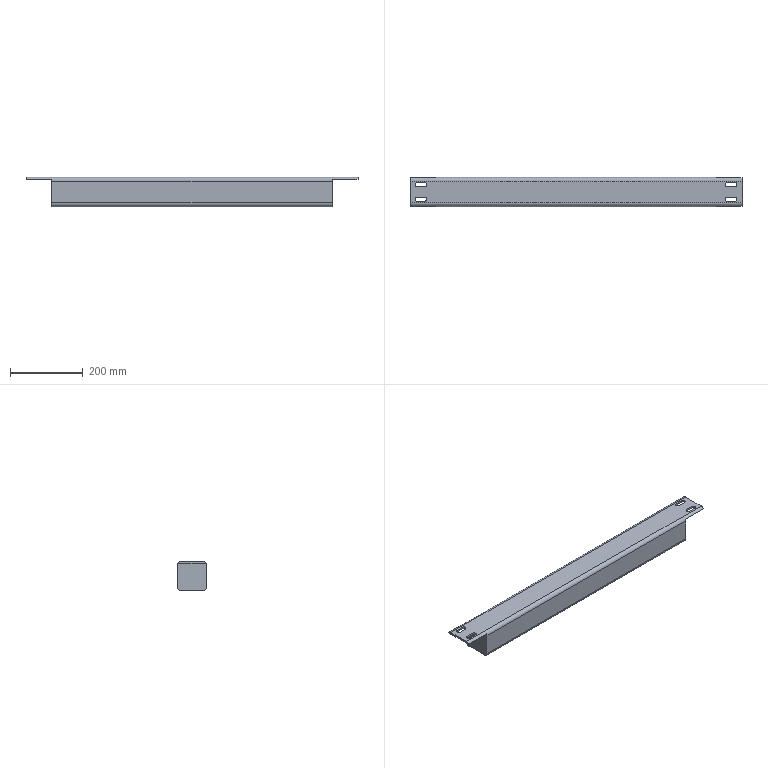Part | SolidWorks | features ICE 3, Extrusion 1, Fillet 1 | 1 solid | 34 faces | box 910 x 80 x 80 mm | volume 4905439 mm3 | plane 18 | cylinder 16 | commonest cylinder face diameters 12 x12 20 x4
STEP:
#1=CARTESIAN_POINT('',(-180.667,10.,35.));
#2=VERTEX_POINT('',#1);
#3=CARTESIAN_POINT('',(-186.667,16.,35.));
#4=VERTEX_POINT('',#3);
#5=CARTESIAN_POINT('',(-186.667,10.,35.));
#6=DIRECTION('',(0.,0.,1.));
#7=DIRECTION('',(1.,0.,0.));
#8=AXIS2_PLACEMENT_3D('',#5,#6,#7);
#9=CIRCLE('',#8,6.);
#10=EDGE_CURVE('',#2,#4,#9,.T.);
#11=ORIENTED_EDGE('',*,*,#10,.F.);
#12=CARTESIAN_POINT('',(-180.667,10.,40.));
#13=VERTEX_POINT('',#12);
#14=CARTESIAN_POINT('',(-180.667,10.,-40.));
#15=DIRECTION('',(0.,0.,1.));
#16=VECTOR('',#15,1000.);
#17=LINE('',#14,#16);
#18=EDGE_CURVE('',#2,#13,#17,.T.);
#19=ORIENTED_EDGE('',*,*,#18,.T.);
#20=CARTESIAN_POINT('',(-186.667,16.,40.));
#21=VERTEX_POINT('',#20);
#22=CARTESIAN_POINT('',(-186.667,10.,40.));
#23=DIRECTION('',(0.,0.,1.));
#24=DIRECTION('',(1.,0.,0.));
#25=AXIS2_PLACEMENT_3D('',#22,#23,#24);
#26=CIRCLE('',#25,6.);
#27=EDGE_CURVE('',#13,#21,#26,.T.);
#28=ORIENTED_EDGE('',*,*,#27,.T.);
#29=CARTESIAN_POINT('',(-186.667,16.,-40.));
#30=DIRECTION('',(0.,0.,1.));
#31=VECTOR('',#30,1000.);
#32=LINE('',#29,#31);
#33=EDGE_CURVE('',#4,#21,#32,.T.);
#34=ORIENTED_EDGE('',*,*,#33,.F.);
#35=EDGE_LOOP('',(#11,#19,#28,#34));
#36=FACE_OUTER_BOUND('',#35,.T.);
#37=CARTESIAN_POINT('',(-186.667,10.,-40.));
#38=DIRECTION('',(0.,0.,1.));
#39=DIRECTION('',(1.,0.,0.));
#40=AXIS2_PLACEMENT_3D('',#37,#38,#39);
#41=CYLINDRICAL_SURFACE('',#40,6.);
#42=ADVANCED_FACE('',(#36),#41,.F.);
#43=CARTESIAN_POINT('',(-180.667,-30.,35.));
#44=VERTEX_POINT('',#43);
#45=CARTESIAN_POINT('',(-186.667,-24.,35.));
#46=VERTEX_POINT('',#45);
#47=CARTESIAN_POINT('',(-186.667,-30.,35.));
#48=DIRECTION('',(0.,0.,1.));
#49=DIRECTION('',(1.,0.,0.));
#50=AXIS2_PLACEMENT_3D('',#47,#48,#49);
#51=CIRCLE('',#50,6.);
#52=EDGE_CURVE('',#44,#46,#51,.T.);
#53=ORIENTED_EDGE('',*,*,#52,.F.);
#54=CARTESIAN_POINT('',(-180.667,-30.,40.));
#55=VERTEX_POINT('',#54);
#56=CARTESIAN_POINT('',(-180.667,-30.,-40.));
#57=DIRECTION('',(0.,0.,1.));
#58=VECTOR('',#57,1000.);
#59=LINE('',#56,#58);
#60=EDGE_CURVE('',#44,#55,#59,.T.);
#61=ORIENTED_EDGE('',*,*,#60,.T.);
#62=CARTESIAN_POINT('',(-186.667,-24.,40.));
#63=VERTEX_POINT('',#62);
#64=CARTESIAN_POINT('',(-186.667,-30.,40.));
#65=DIRECTION('',(0.,0.,1.));
#66=DIRECTION('',(1.,0.,0.));
#67=AXIS2_PLACEMENT_3D('',#64,#65,#66);
#68=CIRCLE('',#67,6.);
#69=EDGE_CURVE('',#55,#63,#68,.T.);
#70=ORIENTED_EDGE('',*,*,#69,.T.);
#71=CARTESIAN_POINT('',(-186.667,-24.,-40.));
#72=DIRECTION('',(0.,0.,1.));
#73=VECTOR('',#72,1000.);
#74=LINE('',#71,#73);
#75=EDGE_CURVE('',#46,#63,#74,.T.);
#76=ORIENTED_EDGE('',*,*,#75,.F.);
#77=EDGE_LOOP('',(#53,#61,#70,#76));
#78=FACE_OUTER_BOUND('',#77,.T.);
#79=CARTESIAN_POINT('',(-186.667,-30.,-40.));
#80=DIRECTION('',(0.,0.,1.));
#81=DIRECTION('',(1.,0.,0.));
#82=AXIS2_PLACEMENT_3D('',#79,#80,#81);
#83=CYLINDRICAL_SURFACE('',#82,6.);
#84=ADVANCED_FACE('',(#78),#83,.F.);
#85=CARTESIAN_POINT('',(669.333,-30.,35.));
#86=VERTEX_POINT('',#85);
#87=CARTESIAN_POINT('',(663.333,-24.,35.));
#88=VERTEX_POINT('',#87);
#89=CARTESIAN_POINT('',(663.333,-30.,35.));
#90=DIRECTION('',(0.,0.,1.));
#91=DIRECTION('',(0.,-1.,0.));
#92=AXIS2_PLACEMENT_3D('',#89,#90,#91);
#93=CIRCLE('',#92,6.);
#94=EDGE_CURVE('',#86,#88,#93,.T.);
#95=ORIENTED_EDGE('',*,*,#94,.F.);
#96=CARTESIAN_POINT('',(669.333,-30.,40.));
#97=VERTEX_POINT('',#96);
#98=CARTESIAN_POINT('',(669.333,-30.,-40.));
#99=DIRECTION('',(0.,0.,1.));
#100=VECTOR('',#99,1000.);
#101=LINE('',#98,#100);
#102=EDGE_CURVE('',#86,#97,#101,.T.);
#103=ORIENTED_EDGE('',*,*,#102,.T.);
#104=CARTESIAN_POINT('',(663.333,-24.,40.));
#105=VERTEX_POINT('',#104);
#106=CARTESIAN_POINT('',(663.333,-30.,40.));
#107=DIRECTION('',(0.,0.,1.));
#108=DIRECTION('',(-1.,0.,0.));
#109=AXIS2_PLACEMENT_3D('',#106,#107,#108);
#110=CIRCLE('',#109,6.);
#111=EDGE_CURVE('',#97,#105,#110,.T.);
#112=ORIENTED_EDGE('',*,*,#111,.T.);
#113=CARTESIAN_POINT('',(663.333,-24.,-40.));
#114=DIRECTION('',(0.,0.,1.));
#115=VECTOR('',#114,1000.);
#116=LINE('',#113,#115);
#117=EDGE_CURVE('',#88,#105,#116,.T.);
#118=ORIENTED_EDGE('',*,*,#117,.F.);
#119=EDGE_LOOP('',(#95,#103,#112,#118));
#120=FACE_OUTER_BOUND('',#119,.T.);
#121=CARTESIAN_POINT('',(663.333,-30.,-40.));
#122=DIRECTION('',(0.,0.,1.));
#123=DIRECTION('',(1.,0.,0.));
#124=AXIS2_PLACEMENT_3D('',#121,#122,#123);
#125=CYLINDRICAL_SURFACE('',#124,6.);
#126=ADVANCED_FACE('',(#120),#125,.F.);
#127=CARTESIAN_POINT('',(669.333,10.,35.));
#128=VERTEX_POINT('',#127);
#129=CARTESIAN_POINT('',(663.333,16.,35.));
#130=VERTEX_POINT('',#129);
#131=CARTESIAN_POINT('',(663.333,10.,35.));
#132=DIRECTION('',(0.,0.,1.));
#133=DIRECTION('',(0.,-1.,0.));
#134=AXIS2_PLACEMENT_3D('',#131,#132,#133);
#135=CIRCLE('',#134,6.);
#136=EDGE_CURVE('',#128,#130,#135,.T.);
#137=ORIENTED_EDGE('',*,*,#136,.F.);
#138=CARTESIAN_POINT('',(669.333,10.,40.));
#139=VERTEX_POINT('',#138);
#140=CARTESIAN_POINT('',(669.333,10.,-40.));
#141=DIRECTION('',(0.,0.,1.));
#142=VECTOR('',#141,1000.);
#143=LINE('',#140,#142);
#144=EDGE_CURVE('',#128,#139,#143,.T.);
#145=ORIENTED_EDGE('',*,*,#144,.T.);
#146=CARTESIAN_POINT('',(663.333,16.,40.));
#147=VERTEX_POINT('',#146);
#148=CARTESIAN_POINT('',(663.333,10.,40.));
#149=DIRECTION('',(0.,0.,1.));
#150=DIRECTION('',(-1.,0.,0.));
#151=AXIS2_PLACEMENT_3D('',#148,#149,#150);
#152=CIRCLE('',#151,6.);
#153=EDGE_CURVE('',#139,#147,#152,.T.);
#154=ORIENTED_EDGE('',*,*,#153,.T.);
#155=CARTESIAN_POINT('',(663.333,16.,-40.));
#156=DIRECTION('',(0.,0.,1.));
#157=VECTOR('',#156,1000.);
#158=LINE('',#155,#157);
#159=EDGE_CURVE('',#130,#147,#158,.T.);
#160=ORIENTED_EDGE('',*,*,#159,.F.);
#161=EDGE_LOOP('',(#137,#145,#154,#160));
#162=FACE_OUTER_BOUND('',#161,.T.);
#163=CARTESIAN_POINT('',(663.333,10.,-40.));
#164=DIRECTION('',(0.,0.,1.));
#165=DIRECTION('',(1.,0.,0.));
#166=AXIS2_PLACEMENT_3D('',#163,#164,#165);
#167=CYLINDRICAL_SURFACE('',#166,6.);
#168=ADVANCED_FACE('',(#162),#167,.F.);
#169=CARTESIAN_POINT('',(613.333,-40.,-40.));
#170=VERTEX_POINT('',#169);
#171=CARTESIAN_POINT('',(613.333,20.,-40.));
#172=VERTEX_POINT('',#171);
#173=CARTESIAN_POINT('',(613.333,-50.,-40.));
#174=DIRECTION('',(0.,1.,0.));
#175=VECTOR('',#174,1000.);
#176=LINE('',#173,#175);
#177=EDGE_CURVE('',#170,#172,#176,.T.);
#178=ORIENTED_EDGE('',*,*,#177,.F.);
#179=CARTESIAN_POINT('',(-156.667,-40.,-40.));
#180=VERTEX_POINT('',#179);
#181=CARTESIAN_POINT('',(-156.667,-40.,-40.));
#182=DIRECTION('',(-1.,0.,0.));
#183=VECTOR('',#182,1000.);
#184=LINE('',#181,#183);
#185=EDGE_CURVE('',#170,#180,#184,.T.);
#186=ORIENTED_EDGE('',*,*,#185,.T.);
#187=CARTESIAN_POINT('',(-156.667,20.,-40.));
#188=VERTEX_POINT('',#187);
#189=CARTESIAN_POINT('',(-156.667,-50.,-40.));
#190=DIRECTION('',(0.,1.,0.));
#191=VECTOR('',#190,1000.);
#192=LINE('',#189,#191);
#193=EDGE_CURVE('',#180,#188,#192,.T.);
#194=ORIENTED_EDGE('',*,*,#193,.T.);
#195=CARTESIAN_POINT('',(613.333,20.,-40.));
#196=DIRECTION('',(1.,0.,0.));
#197=VECTOR('',#196,1000.);
#198=LINE('',#195,#197);
#199=EDGE_CURVE('',#188,#172,#198,.T.);
#200=ORIENTED_EDGE('',*,*,#199,.T.);
#201=EDGE_LOOP('',(#178,#186,#194,#200));
#202=FACE_OUTER_BOUND('',#201,.T.);
#203=CARTESIAN_POINT('',(613.333,-50.,-40.));
#204=DIRECTION('',(0.,0.,-1.));
#205=DIRECTION('',(-1.,0.,0.));
#206=AXIS2_PLACEMENT_3D('',#203,#204,#205);
#207=PLANE('',#206);
#208=ADVANCED_FACE('',(#202),#207,.T.);
#209=CARTESIAN_POINT('',(613.333,30.,30.));
#210=VERTEX_POINT('',#209);
#211=CARTESIAN_POINT('',(613.333,30.,-30.));
#212=VERTEX_POINT('',#211);
#213=CARTESIAN_POINT('',(613.333,30.,40.));
#214=DIRECTION('',(0.,0.,-1.));
#215=VECTOR('',#214,1000.);
#216=LINE('',#213,#215);
#217=EDGE_CURVE('',#210,#212,#216,.T.);
#218=ORIENTED_EDGE('',*,*,#217,.F.);
#219=CARTESIAN_POINT('',(613.333,28.66,35.));
#220=VERTEX_POINT('',#219);
#221=CARTESIAN_POINT('',(613.333,20.,30.));
#222=DIRECTION('',(1.,0.,0.));
#223=DIRECTION('',(0.,0.,-1.));
#224=AXIS2_PLACEMENT_3D('',#221,#222,#223);
#225=CIRCLE('',#224,10.);
#226=EDGE_CURVE('',#210,#220,#225,.T.);
#227=ORIENTED_EDGE('',*,*,#226,.T.);
#228=CARTESIAN_POINT('',(613.333,-48.66,35.));
#229=VERTEX_POINT('',#228);
#230=CARTESIAN_POINT('',(613.333,30.,35.));
#231=DIRECTION('',(0.,1.,0.));
#232=VECTOR('',#231,1000.);
#233=LINE('',#230,#232);
#234=EDGE_CURVE('',#229,#220,#233,.T.);
#235=ORIENTED_EDGE('',*,*,#234,.F.);
#236=CARTESIAN_POINT('',(613.333,-50.,30.));
#237=VERTEX_POINT('',#236);
#238=CARTESIAN_POINT('',(613.333,-40.,30.));
#239=DIRECTION('',(1.,0.,0.));
#240=DIRECTION('',(0.,0.,-1.));
#241=AXIS2_PLACEMENT_3D('',#238,#239,#240);
#242=CIRCLE('',#241,10.);
#243=EDGE_CURVE('',#229,#237,#242,.T.);
#244=ORIENTED_EDGE('',*,*,#243,.T.);
#245=CARTESIAN_POINT('',(613.333,-50.,-30.));
#246=VERTEX_POINT('',#245);
#247=CARTESIAN_POINT('',(613.333,-50.,40.));
#248=DIRECTION('',(0.,0.,-1.));
#249=VECTOR('',#248,1000.);
#250=LINE('',#247,#249);
#251=EDGE_CURVE('',#237,#246,#250,.T.);
#252=ORIENTED_EDGE('',*,*,#251,.T.);
#253=CARTESIAN_POINT('',(613.333,-40.,-30.));
#254=DIRECTION('',(1.,0.,0.));
#255=DIRECTION('',(0.,0.,-1.));
#256=AXIS2_PLACEMENT_3D('',#253,#254,#255);
#257=CIRCLE('',#256,10.);
#258=EDGE_CURVE('',#246,#170,#257,.T.);
#259=ORIENTED_EDGE('',*,*,#258,.T.);
#260=ORIENTED_EDGE('',*,*,#177,.T.);
#261=CARTESIAN_POINT('',(613.333,20.,-30.));
#262=DIRECTION('',(1.,0.,0.));
#263=DIRECTION('',(0.,0.,-1.));
#264=AXIS2_PLACEMENT_3D('',#261,#262,#263);
#265=CIRCLE('',#264,10.);
#266=EDGE_CURVE('',#172,#212,#265,.T.);
#267=ORIENTED_EDGE('',*,*,#266,.T.);
#268=EDGE_LOOP('',(#218,#227,#235,#244,#252,#259,#260,#267));
#269=FACE_OUTER_BOUND('',#268,.T.);
#270=CARTESIAN_POINT('',(613.333,-50.,40.));
#271=DIRECTION('',(1.,0.,0.));
#272=DIRECTION('',(0.,0.,-1.));
#273=AXIS2_PLACEMENT_3D('',#270,#271,#272);
#274=PLANE('',#273);
#275=ADVANCED_FACE('',(#269),#274,.T.);
#276=CARTESIAN_POINT('',(663.333,-36.,40.));
#277=VERTEX_POINT('',#276);
#278=CARTESIAN_POINT('',(663.333,-30.,40.));
#279=DIRECTION('',(0.,0.,1.));
#280=DIRECTION('',(-1.,0.,0.));
#281=AXIS2_PLACEMENT_3D('',#278,#279,#280);
#282=CIRCLE('',#281,6.);
#283=EDGE_CURVE('',#277,#97,#282,.T.);
#284=ORIENTED_EDGE('',*,*,#283,.F.);
#285=CARTESIAN_POINT('',(643.333,-36.,40.));
#286=VERTEX_POINT('',#285);
#287=CARTESIAN_POINT('',(663.333,-36.,40.));
#288=DIRECTION('',(1.,0.,0.));
#289=VECTOR('',#288,1000.);
#290=LINE('',#287,#289);
#291=EDGE_CURVE('',#286,#277,#290,.T.);
#292=ORIENTED_EDGE('',*,*,#291,.F.);
#293=CARTESIAN_POINT('',(643.333,-24.,40.));
#294=VERTEX_POINT('',#293);
#295=CARTESIAN_POINT('',(643.333,-30.,40.));
#296=DIRECTION('',(0.,0.,1.));
#297=DIRECTION('',(-1.,0.,0.));
#298=AXIS2_PLACEMENT_3D('',#295,#296,#297);
#299=CIRCLE('',#298,6.);
#300=EDGE_CURVE('',#294,#286,#299,.T.);
#301=ORIENTED_EDGE('',*,*,#300,.F.);
#302=CARTESIAN_POINT('',(663.333,-24.,40.));
#303=DIRECTION('',(-1.,0.,0.));
#304=VECTOR('',#303,1000.);
#305=LINE('',#302,#304);
#306=EDGE_CURVE('',#105,#294,#305,.T.);
#307=ORIENTED_EDGE('',*,*,#306,.F.);
#308=ORIENTED_EDGE('',*,*,#111,.F.);
#309=EDGE_LOOP('',(#284,#292,#301,#307,#308));
#310=FACE_BOUND('',#309,.T.);
#311=CARTESIAN_POINT('',(663.333,4.,40.));
#312=VERTEX_POINT('',#311);
#313=CARTESIAN_POINT('',(663.333,10.,40.));
#314=DIRECTION('',(0.,0.,1.));
#315=DIRECTION('',(-1.,0.,0.));
#316=AXIS2_PLACEMENT_3D('',#313,#314,#315);
#317=CIRCLE('',#316,6.);
#318=EDGE_CURVE('',#312,#139,#317,.T.);
#319=ORIENTED_EDGE('',*,*,#318,.F.);
#320=CARTESIAN_POINT('',(643.333,4.,40.));
#321=VERTEX_POINT('',#320);
#322=CARTESIAN_POINT('',(663.333,4.,40.));
#323=DIRECTION('',(1.,0.,0.));
#324=VECTOR('',#323,1000.);
#325=LINE('',#322,#324);
#326=EDGE_CURVE('',#321,#312,#325,.T.);
#327=ORIENTED_EDGE('',*,*,#326,.F.);
#328=CARTESIAN_POINT('',(643.333,16.,40.));
#329=VERTEX_POINT('',#328);
#330=CARTESIAN_POINT('',(643.333,10.,40.));
#331=DIRECTION('',(0.,0.,1.));
#332=DIRECTION('',(-1.,0.,0.));
#333=AXIS2_PLACEMENT_3D('',#330,#331,#332);
#334=CIRCLE('',#333,6.);
#335=EDGE_CURVE('',#329,#321,#334,.T.);
#336=ORIENTED_EDGE('',*,*,#335,.F.);
#337=CARTESIAN_POINT('',(663.333,16.,40.));
#338=DIRECTION('',(-1.,0.,0.));
#339=VECTOR('',#338,1000.);
#340=LINE('',#337,#339);
#341=EDGE_CURVE('',#147,#329,#340,.T.);
#342=ORIENTED_EDGE('',*,*,#341,.F.);
#343=ORIENTED_EDGE('',*,*,#153,.F.);
#344=EDGE_LOOP('',(#319,#327,#336,#342,#343));
#345=FACE_BOUND('',#344,.T.);
#346=CARTESIAN_POINT('',(-206.667,16.,40.));
#347=VERTEX_POINT('',#346);
#348=CARTESIAN_POINT('',(-206.667,4.,40.));
#349=VERTEX_POINT('',#348);
#350=CARTESIAN_POINT('',(-206.667,10.,40.));
#351=DIRECTION('',(0.,0.,1.));
#352=DIRECTION('',(1.,0.,0.));
#353=AXIS2_PLACEMENT_3D('',#350,#351,#352);
#354=CIRCLE('',#353,6.);
#355=EDGE_CURVE('',#347,#349,#354,.T.);
#356=ORIENTED_EDGE('',*,*,#355,.F.);
#357=CARTESIAN_POINT('',(-206.667,16.,40.));
#358=DIRECTION('',(-1.,0.,0.));
#359=VECTOR('',#358,1000.);
#360=LINE('',#357,#359);
#361=EDGE_CURVE('',#21,#347,#360,.T.);
#362=ORIENTED_EDGE('',*,*,#361,.F.);
#363=ORIENTED_EDGE('',*,*,#27,.F.);
#364=CARTESIAN_POINT('',(-186.667,4.,40.));
#365=VERTEX_POINT('',#364);
#366=CARTESIAN_POINT('',(-186.667,10.,40.));
#367=DIRECTION('',(0.,0.,1.));
#368=DIRECTION('',(1.,0.,0.));
#369=AXIS2_PLACEMENT_3D('',#366,#367,#368);
#370=CIRCLE('',#369,6.);
#371=EDGE_CURVE('',#365,#13,#370,.T.);
#372=ORIENTED_EDGE('',*,*,#371,.F.);
#373=CARTESIAN_POINT('',(-206.667,4.,40.));
#374=DIRECTION('',(1.,0.,0.));
#375=VECTOR('',#374,1000.);
#376=LINE('',#373,#375);
#377=EDGE_CURVE('',#349,#365,#376,.T.);
#378=ORIENTED_EDGE('',*,*,#377,.F.);
#379=EDGE_LOOP('',(#356,#362,#363,#372,#378));
#380=FACE_BOUND('',#379,.T.);
#381=CARTESIAN_POINT('',(-206.667,-24.,40.));
#382=VERTEX_POINT('',#381);
#383=CARTESIAN_POINT('',(-206.667,-36.,40.));
#384=VERTEX_POINT('',#383);
#385=CARTESIAN_POINT('',(-206.667,-30.,40.));
#386=DIRECTION('',(0.,0.,1.));
#387=DIRECTION('',(1.,0.,0.));
#388=AXIS2_PLACEMENT_3D('',#385,#386,#387);
#389=CIRCLE('',#388,6.);
#390=EDGE_CURVE('',#382,#384,#389,.T.);
#391=ORIENTED_EDGE('',*,*,#390,.F.);
#392=CARTESIAN_POINT('',(-206.667,-24.,40.));
#393=DIRECTION('',(-1.,0.,0.));
#394=VECTOR('',#393,1000.);
#395=LINE('',#392,#394);
#396=EDGE_CURVE('',#63,#382,#395,.T.);
#397=ORIENTED_EDGE('',*,*,#396,.F.);
#398=ORIENTED_EDGE('',*,*,#69,.F.);
#399=CARTESIAN_POINT('',(-186.667,-36.,40.));
#400=VERTEX_POINT('',#399);
#401=CARTESIAN_POINT('',(-186.667,-30.,40.));
#402=DIRECTION('',(0.,0.,1.));
#403=DIRECTION('',(1.,0.,0.));
#404=AXIS2_PLACEMENT_3D('',#401,#402,#403);
#405=CIRCLE('',#404,6.);
#406=EDGE_CURVE('',#400,#55,#405,.T.);
#407=ORIENTED_EDGE('',*,*,#406,.F.);
#408=CARTESIAN_POINT('',(-206.667,-36.,40.));
#409=DIRECTION('',(1.,0.,0.));
#410=VECTOR('',#409,1000.);
#411=LINE('',#408,#410);
#412=EDGE_CURVE('',#384,#400,#411,.T.);
#413=ORIENTED_EDGE('',*,*,#412,.F.);
#414=EDGE_LOOP('',(#391,#397,#398,#407,#413));
#415=FACE_BOUND('',#414,.T.);
#416=CARTESIAN_POINT('',(683.333,20.,40.));
#417=VERTEX_POINT('',#416);
#418=CARTESIAN_POINT('',(683.333,-40.,40.));
#419=VERTEX_POINT('',#418);
#420=CARTESIAN_POINT('',(683.333,-50.,40.));
#421=DIRECTION('',(0.,-1.,0.));
#422=VECTOR('',#421,1000.);
#423=LINE('',#420,#422);
#424=EDGE_CURVE('',#417,#419,#423,.T.);
#425=ORIENTED_EDGE('',*,*,#424,.F.);
#426=CARTESIAN_POINT('',(-226.667,20.,40.));
#427=VERTEX_POINT('',#426);
#428=CARTESIAN_POINT('',(-156.667,20.,40.));
#429=DIRECTION('',(-1.,0.,0.));
#430=VECTOR('',#429,1000.);
#431=LINE('',#428,#430);
#432=EDGE_CURVE('',#417,#427,#431,.T.);
#433=ORIENTED_EDGE('',*,*,#432,.T.);
#434=CARTESIAN_POINT('',(-226.667,-40.,40.));
#435=VERTEX_POINT('',#434);
#436=CARTESIAN_POINT('',(-226.667,30.,40.));
#437=DIRECTION('',(0.,1.,0.));
#438=VECTOR('',#437,1000.);
#439=LINE('',#436,#438);
#440=EDGE_CURVE('',#435,#427,#439,.T.);
#441=ORIENTED_EDGE('',*,*,#440,.F.);
#442=CARTESIAN_POINT('',(683.333,-40.,40.));
#443=DIRECTION('',(1.,0.,0.));
#444=VECTOR('',#443,1000.);
#445=LINE('',#442,#444);
#446=EDGE_CURVE('',#435,#419,#445,.T.);
#447=ORIENTED_EDGE('',*,*,#446,.T.);
#448=EDGE_LOOP('',(#425,#433,#441,#447));
#449=FACE_OUTER_BOUND('',#448,.T.);
#450=CARTESIAN_POINT('',(-156.667,-50.,40.));
#451=DIRECTION('',(0.,0.,1.));
#452=DIRECTION('',(1.,0.,0.));
#453=AXIS2_PLACEMENT_3D('',#450,#451,#452);
#454=PLANE('',#453);
#455=ADVANCED_FACE('',(#310,#345,#380,#415,#449),#454,.T.);
#456=CARTESIAN_POINT('',(-156.667,28.66,35.));
#457=VERTEX_POINT('',#456);
#458=CARTESIAN_POINT('',(-156.667,-48.66,35.));
#459=VERTEX_POINT('',#458);
#460=CARTESIAN_POINT('',(-156.667,-50.,35.));
#461=DIRECTION('',(0.,-1.,0.));
#462=VECTOR('',#461,1000.);
#463=LINE('',#460,#462);
#464=EDGE_CURVE('',#457,#459,#463,.T.);
#465=ORIENTED_EDGE('',*,*,#464,.F.);
#466=CARTESIAN_POINT('',(-156.667,30.,30.));
#467=VERTEX_POINT('',#466);
#468=CARTESIAN_POINT('',(-156.667,20.,30.));
#469=DIRECTION('',(-1.,0.,0.));
#470=DIRECTION('',(0.,0.,1.));
#471=AXIS2_PLACEMENT_3D('',#468,#469,#470);
#472=CIRCLE('',#471,10.);
#473=EDGE_CURVE('',#457,#467,#472,.T.);
#474=ORIENTED_EDGE('',*,*,#473,.T.);
#475=CARTESIAN_POINT('',(-156.667,30.,-30.));
#476=VERTEX_POINT('',#475);
#477=CARTESIAN_POINT('',(-156.667,30.,-40.));
#478=DIRECTION('',(0.,0.,1.));
#479=VECTOR('',#478,1000.);
#480=LINE('',#477,#479);
#481=EDGE_CURVE('',#476,#467,#480,.T.);
#482=ORIENTED_EDGE('',*,*,#481,.F.);
#483=CARTESIAN_POINT('',(-156.667,20.,-30.));
#484=DIRECTION('',(-1.,0.,0.));
#485=DIRECTION('',(0.,0.,1.));
#486=AXIS2_PLACEMENT_3D('',#483,#484,#485);
#487=CIRCLE('',#486,10.);
#488=EDGE_CURVE('',#476,#188,#487,.T.);
#489=ORIENTED_EDGE('',*,*,#488,.T.);
#490=ORIENTED_EDGE('',*,*,#193,.F.);
#491=CARTESIAN_POINT('',(-156.667,-50.,-30.));
#492=VERTEX_POINT('',#491);
#493=CARTESIAN_POINT('',(-156.667,-40.,-30.));
#494=DIRECTION('',(-1.,0.,0.));
#495=DIRECTION('',(0.,0.,1.));
#496=AXIS2_PLACEMENT_3D('',#493,#494,#495);
#497=CIRCLE('',#496,10.);
#498=EDGE_CURVE('',#180,#492,#497,.T.);
#499=ORIENTED_EDGE('',*,*,#498,.T.);
#500=CARTESIAN_POINT('',(-156.667,-50.,30.));
#501=VERTEX_POINT('',#500);
#502=CARTESIAN_POINT('',(-156.667,-50.,-40.));
#503=DIRECTION('',(0.,0.,1.));
#504=VECTOR('',#503,1000.);
#505=LINE('',#502,#504);
#506=EDGE_CURVE('',#492,#501,#505,.T.);
#507=ORIENTED_EDGE('',*,*,#506,.T.);
#508=CARTESIAN_POINT('',(-156.667,-40.,30.));
#509=DIRECTION('',(-1.,0.,0.));
#510=DIRECTION('',(0.,0.,1.));
#511=AXIS2_PLACEMENT_3D('',#508,#509,#510);
#512=CIRCLE('',#511,10.);
#513=EDGE_CURVE('',#501,#459,#512,.T.);
#514=ORIENTED_EDGE('',*,*,#513,.T.);
#515=EDGE_LOOP('',(#465,#474,#482,#489,#490,#499,#507,#514));
#516=FACE_OUTER_BOUND('',#515,.T.);
#517=CARTESIAN_POINT('',(-156.667,-50.,-40.));
#518=DIRECTION('',(-1.,0.,0.));
#519=DIRECTION('',(0.,0.,1.));
#520=AXIS2_PLACEMENT_3D('',#517,#518,#519);
#521=PLANE('',#520);
#522=ADVANCED_FACE('',(#516),#521,.T.);
#523=ORIENTED_EDGE('',*,*,#251,.F.);
#524=CARTESIAN_POINT('',(-226.667,-50.,30.));
#525=DIRECTION('',(-1.,0.,0.));
#526=VECTOR('',#525,1000.);
#527=LINE('',#524,#526);
#528=EDGE_CURVE('',#237,#501,#527,.T.);
#529=ORIENTED_EDGE('',*,*,#528,.T.);
#530=ORIENTED_EDGE('',*,*,#506,.F.);
#531=CARTESIAN_POINT('',(613.333,-50.,-30.));
#532=DIRECTION('',(1.,0.,0.));
#533=VECTOR('',#532,1000.);
#534=LINE('',#531,#533);
#535=EDGE_CURVE('',#492,#246,#534,.T.);
#536=ORIENTED_EDGE('',*,*,#535,.T.);
#537=EDGE_LOOP('',(#523,#529,#530,#536));
#538=FACE_OUTER_BOUND('',#537,.T.);
#539=CARTESIAN_POINT('',(0.,-50.,0.));
#540=DIRECTION('',(0.,1.,0.));
#541=DIRECTION('',(0.,0.,1.));
#542=AXIS2_PLACEMENT_3D('',#539,#540,#541);
#543=PLANE('',#542);
#544=ADVANCED_FACE('',(#538),#543,.F.);
#545=ORIENTED_EDGE('',*,*,#481,.T.);
#546=CARTESIAN_POINT('',(0.,30.,30.));
#547=DIRECTION('',(1.,0.,0.));
#548=VECTOR('',#547,1000.);
#549=LINE('',#546,#548);
#550=EDGE_CURVE('',#467,#210,#549,.T.);
#551=ORIENTED_EDGE('',*,*,#550,.T.);
#552=ORIENTED_EDGE('',*,*,#217,.T.);
#553=CARTESIAN_POINT('',(0.,30.,-30.));
#554=DIRECTION('',(-1.,0.,0.));
#555=VECTOR('',#554,1000.);
#556=LINE('',#553,#555);
#557=EDGE_CURVE('',#212,#476,#556,.T.);
#558=ORIENTED_EDGE('',*,*,#557,.T.);
#559=EDGE_LOOP('',(#545,#551,#552,#558));
#560=FACE_OUTER_BOUND('',#559,.T.);
#561=CARTESIAN_POINT('',(0.,30.,0.));
#562=DIRECTION('',(0.,1.,0.));
#563=DIRECTION('',(0.,0.,1.));
#564=AXIS2_PLACEMENT_3D('',#561,#562,#563);
#565=PLANE('',#564);
#566=ADVANCED_FACE('',(#560),#565,.T.);
#567=CARTESIAN_POINT('',(-206.667,16.,35.));
#568=VERTEX_POINT('',#567);
#569=CARTESIAN_POINT('',(-226.667,16.,35.));
#570=DIRECTION('',(-1.,0.,0.));
#571=VECTOR('',#570,1000.);
#572=LINE('',#569,#571);
#573=EDGE_CURVE('',#4,#568,#572,.T.);
#574=ORIENTED_EDGE('',*,*,#573,.T.);
#575=CARTESIAN_POINT('',(-206.667,4.,35.));
#576=VERTEX_POINT('',#575);
#577=CARTESIAN_POINT('',(-206.667,10.,35.));
#578=DIRECTION('',(0.,0.,1.));
#579=DIRECTION('',(1.,0.,0.));
#580=AXIS2_PLACEMENT_3D('',#577,#578,#579);
#581=CIRCLE('',#580,6.);
#582=EDGE_CURVE('',#568,#576,#581,.T.);
#583=ORIENTED_EDGE('',*,*,#582,.T.);
#584=CARTESIAN_POINT('',(-186.667,4.,35.));
#585=VERTEX_POINT('',#584);
#586=CARTESIAN_POINT('',(-226.667,4.,35.));
#587=DIRECTION('',(1.,0.,0.));
#588=VECTOR('',#587,1000.);
#589=LINE('',#586,#588);
#590=EDGE_CURVE('',#576,#585,#589,.T.);
#591=ORIENTED_EDGE('',*,*,#590,.T.);
#592=CARTESIAN_POINT('',(-186.667,10.,35.));
#593=DIRECTION('',(0.,0.,1.));
#594=DIRECTION('',(1.,0.,0.));
#595=AXIS2_PLACEMENT_3D('',#592,#593,#594);
#596=CIRCLE('',#595,6.);
#597=EDGE_CURVE('',#585,#2,#596,.T.);
#598=ORIENTED_EDGE('',*,*,#597,.T.);
#599=ORIENTED_EDGE('',*,*,#10,.T.);
#600=EDGE_LOOP('',(#574,#583,#591,#598,#599));
#601=FACE_BOUND('',#600,.T.);
#602=CARTESIAN_POINT('',(-206.667,-24.,35.));
#603=VERTEX_POINT('',#602);
#604=CARTESIAN_POINT('',(-226.667,-24.,35.));
#605=DIRECTION('',(-1.,0.,0.));
#606=VECTOR('',#605,1000.);
#607=LINE('',#604,#606);
#608=EDGE_CURVE('',#46,#603,#607,.T.);
#609=ORIENTED_EDGE('',*,*,#608,.T.);
#610=CARTESIAN_POINT('',(-206.667,-36.,35.));
#611=VERTEX_POINT('',#610);
#612=CARTESIAN_POINT('',(-206.667,-30.,35.));
#613=DIRECTION('',(0.,0.,1.));
#614=DIRECTION('',(1.,0.,0.));
#615=AXIS2_PLACEMENT_3D('',#612,#613,#614);
#616=CIRCLE('',#615,6.);
#617=EDGE_CURVE('',#603,#611,#616,.T.);
#618=ORIENTED_EDGE('',*,*,#617,.T.);
#619=CARTESIAN_POINT('',(-186.667,-36.,35.));
#620=VERTEX_POINT('',#619);
#621=CARTESIAN_POINT('',(-226.667,-36.,35.));
#622=DIRECTION('',(1.,0.,0.));
#623=VECTOR('',#622,1000.);
#624=LINE('',#621,#623);
#625=EDGE_CURVE('',#611,#620,#624,.T.);
#626=ORIENTED_EDGE('',*,*,#625,.T.);
#627=CARTESIAN_POINT('',(-186.667,-30.,35.));
#628=DIRECTION('',(0.,0.,1.));
#629=DIRECTION('',(1.,0.,0.));
#630=AXIS2_PLACEMENT_3D('',#627,#628,#629);
#631=CIRCLE('',#630,6.);
#632=EDGE_CURVE('',#620,#44,#631,.T.);
#633=ORIENTED_EDGE('',*,*,#632,.T.);
#634=ORIENTED_EDGE('',*,*,#52,.T.);
#635=EDGE_LOOP('',(#609,#618,#626,#633,#634));
#636=FACE_BOUND('',#635,.T.);
#637=CARTESIAN_POINT('',(-226.667,28.66,35.));
#638=VERTEX_POINT('',#637);
#639=CARTESIAN_POINT('',(-226.667,-48.66,35.));
#640=VERTEX_POINT('',#639);
#641=CARTESIAN_POINT('',(-226.667,-50.,35.));
#642=DIRECTION('',(0.,-1.,0.));
#643=VECTOR('',#642,1000.);
#644=LINE('',#641,#643);
#645=EDGE_CURVE('',#638,#640,#644,.T.);
#646=ORIENTED_EDGE('',*,*,#645,.F.);
#647=CARTESIAN_POINT('',(-226.667,28.66,35.));
#648=DIRECTION('',(1.,0.,0.));
#649=VECTOR('',#648,1000.);
#650=LINE('',#647,#649);
#651=EDGE_CURVE('',#638,#457,#650,.T.);
#652=ORIENTED_EDGE('',*,*,#651,.T.);
#653=ORIENTED_EDGE('',*,*,#464,.T.);
#654=CARTESIAN_POINT('',(-156.667,-48.66,35.));
#655=DIRECTION('',(-1.,0.,0.));
#656=VECTOR('',#655,1000.);
#657=LINE('',#654,#656);
#658=EDGE_CURVE('',#459,#640,#657,.T.);
#659=ORIENTED_EDGE('',*,*,#658,.T.);
#660=EDGE_LOOP('',(#646,#652,#653,#659));
#661=FACE_OUTER_BOUND('',#660,.T.);
#662=CARTESIAN_POINT('',(-226.667,-50.,35.));
#663=DIRECTION('',(0.,0.,1.));
#664=DIRECTION('',(1.,0.,0.));
#665=AXIS2_PLACEMENT_3D('',#662,#663,#664);
#666=PLANE('',#665);
#667=ADVANCED_FACE('',(#601,#636,#661),#666,.F.);
#668=ORIENTED_EDGE('',*,*,#440,.T.);
#669=CARTESIAN_POINT('',(-226.667,20.,30.));
#670=DIRECTION('',(-1.,0.,0.));
#671=DIRECTION('',(0.,0.,-1.));
#672=AXIS2_PLACEMENT_3D('',#669,#670,#671);
#673=CIRCLE('',#672,10.);
#674=EDGE_CURVE('',#427,#638,#673,.T.);
#675=ORIENTED_EDGE('',*,*,#674,.T.);
#676=ORIENTED_EDGE('',*,*,#645,.T.);
#677=CARTESIAN_POINT('',(-226.667,-40.,30.));
#678=DIRECTION('',(-1.,0.,0.));
#679=DIRECTION('',(0.,0.,-1.));
#680=AXIS2_PLACEMENT_3D('',#677,#678,#679);
#681=CIRCLE('',#680,10.);
#682=EDGE_CURVE('',#640,#435,#681,.T.);
#683=ORIENTED_EDGE('',*,*,#682,.T.);
#684=EDGE_LOOP('',(#668,#675,#676,#683));
#685=FACE_OUTER_BOUND('',#684,.T.);
#686=CARTESIAN_POINT('',(-226.667,0.,0.));
#687=DIRECTION('',(1.,0.,0.));
#688=DIRECTION('',(0.,0.,-1.));
#689=AXIS2_PLACEMENT_3D('',#686,#687,#688);
#690=PLANE('',#689);
#691=ADVANCED_FACE('',(#685),#690,.F.);
#692=CARTESIAN_POINT('',(643.333,-36.,35.));
#693=VERTEX_POINT('',#692);
#694=CARTESIAN_POINT('',(663.333,-36.,35.));
#695=VERTEX_POINT('',#694);
#696=CARTESIAN_POINT('',(683.333,-36.,35.));
#697=DIRECTION('',(1.,0.,0.));
#698=VECTOR('',#697,1000.);
#699=LINE('',#696,#698);
#700=EDGE_CURVE('',#693,#695,#699,.T.);
#701=ORIENTED_EDGE('',*,*,#700,.T.);
#702=CARTESIAN_POINT('',(663.333,-30.,35.));
#703=DIRECTION('',(0.,0.,1.));
#704=DIRECTION('',(0.,-1.,0.));
#705=AXIS2_PLACEMENT_3D('',#702,#703,#704);
#706=CIRCLE('',#705,6.);
#707=EDGE_CURVE('',#695,#86,#706,.T.);
#708=ORIENTED_EDGE('',*,*,#707,.T.);
#709=ORIENTED_EDGE('',*,*,#94,.T.);
#710=CARTESIAN_POINT('',(643.333,-24.,35.));
#711=VERTEX_POINT('',#710);
#712=CARTESIAN_POINT('',(683.333,-24.,35.));
#713=DIRECTION('',(-1.,0.,0.));
#714=VECTOR('',#713,1000.);
#715=LINE('',#712,#714);
#716=EDGE_CURVE('',#88,#711,#715,.T.);
#717=ORIENTED_EDGE('',*,*,#716,.T.);
#718=CARTESIAN_POINT('',(643.333,-30.,35.));
#719=DIRECTION('',(0.,0.,1.));
#720=DIRECTION('',(0.,-1.,0.));
#721=AXIS2_PLACEMENT_3D('',#718,#719,#720);
#722=CIRCLE('',#721,6.);
#723=EDGE_CURVE('',#711,#693,#722,.T.);
#724=ORIENTED_EDGE('',*,*,#723,.T.);
#725=EDGE_LOOP('',(#701,#708,#709,#717,#724));
#726=FACE_BOUND('',#725,.T.);
#727=CARTESIAN_POINT('',(643.333,4.,35.));
#728=VERTEX_POINT('',#727);
#729=CARTESIAN_POINT('',(663.333,4.,35.));
#730=VERTEX_POINT('',#729);
#731=CARTESIAN_POINT('',(683.333,4.,35.));
#732=DIRECTION('',(1.,0.,0.));
#733=VECTOR('',#732,1000.);
#734=LINE('',#731,#733);
#735=EDGE_CURVE('',#728,#730,#734,.T.);
#736=ORIENTED_EDGE('',*,*,#735,.T.);
#737=CARTESIAN_POINT('',(663.333,10.,35.));
#738=DIRECTION('',(0.,0.,1.));
#739=DIRECTION('',(0.,-1.,0.));
#740=AXIS2_PLACEMENT_3D('',#737,#738,#739);
#741=CIRCLE('',#740,6.);
#742=EDGE_CURVE('',#730,#128,#741,.T.);
#743=ORIENTED_EDGE('',*,*,#742,.T.);
#744=ORIENTED_EDGE('',*,*,#136,.T.);
#745=CARTESIAN_POINT('',(643.333,16.,35.));
#746=VERTEX_POINT('',#745);
#747=CARTESIAN_POINT('',(683.333,16.,35.));
#748=DIRECTION('',(-1.,0.,0.));
#749=VECTOR('',#748,1000.);
#750=LINE('',#747,#749);
#751=EDGE_CURVE('',#130,#746,#750,.T.);
#752=ORIENTED_EDGE('',*,*,#751,.T.);
#753=CARTESIAN_POINT('',(643.333,10.,35.));
#754=DIRECTION('',(0.,0.,1.));
#755=DIRECTION('',(0.,-1.,0.));
#756=AXIS2_PLACEMENT_3D('',#753,#754,#755);
#757=CIRCLE('',#756,6.);
#758=EDGE_CURVE('',#746,#728,#757,.T.);
#759=ORIENTED_EDGE('',*,*,#758,.T.);
#760=EDGE_LOOP('',(#736,#743,#744,#752,#759));
#761=FACE_BOUND('',#760,.T.);
#762=ORIENTED_EDGE('',*,*,#234,.T.);
#763=CARTESIAN_POINT('',(683.333,28.66,35.));
#764=VERTEX_POINT('',#763);
#765=CARTESIAN_POINT('',(613.333,28.66,35.));
#766=DIRECTION('',(1.,0.,0.));
#767=VECTOR('',#766,1000.);
#768=LINE('',#765,#767);
#769=EDGE_CURVE('',#220,#764,#768,.T.);
#770=ORIENTED_EDGE('',*,*,#769,.T.);
#771=CARTESIAN_POINT('',(683.333,-48.66,35.));
#772=VERTEX_POINT('',#771);
#773=CARTESIAN_POINT('',(683.333,30.,35.));
#774=DIRECTION('',(0.,1.,0.));
#775=VECTOR('',#774,1000.);
#776=LINE('',#773,#775);
#777=EDGE_CURVE('',#772,#764,#776,.T.);
#778=ORIENTED_EDGE('',*,*,#777,.F.);
#779=CARTESIAN_POINT('',(683.333,-48.66,35.));
#780=DIRECTION('',(-1.,0.,0.));
#781=VECTOR('',#780,1000.);
#782=LINE('',#779,#781);
#783=EDGE_CURVE('',#772,#229,#782,.T.);
#784=ORIENTED_EDGE('',*,*,#783,.T.);
#785=EDGE_LOOP('',(#762,#770,#778,#784));
#786=FACE_OUTER_BOUND('',#785,.T.);
#787=CARTESIAN_POINT('',(683.333,30.,35.));
#788=DIRECTION('',(0.,0.,1.));
#789=DIRECTION('',(0.,-1.,0.));
#790=AXIS2_PLACEMENT_3D('',#787,#788,#789);
#791=PLANE('',#790);
#792=ADVANCED_FACE('',(#726,#761,#786),#791,.F.);
#793=ORIENTED_EDGE('',*,*,#777,.T.);
#794=CARTESIAN_POINT('',(683.333,20.,30.));
#795=DIRECTION('',(1.,0.,0.));
#796=DIRECTION('',(0.,0.,1.));
#797=AXIS2_PLACEMENT_3D('',#794,#795,#796);
#798=CIRCLE('',#797,10.);
#799=EDGE_CURVE('',#764,#417,#798,.T.);
#800=ORIENTED_EDGE('',*,*,#799,.T.);
#801=ORIENTED_EDGE('',*,*,#424,.T.);
#802=CARTESIAN_POINT('',(683.333,-40.,30.));
#803=DIRECTION('',(1.,0.,0.));
#804=DIRECTION('',(0.,0.,1.));
#805=AXIS2_PLACEMENT_3D('',#802,#803,#804);
#806=CIRCLE('',#805,10.);
#807=EDGE_CURVE('',#419,#772,#806,.T.);
#808=ORIENTED_EDGE('',*,*,#807,.T.);
#809=EDGE_LOOP('',(#793,#800,#801,#808));
#810=FACE_OUTER_BOUND('',#809,.T.);
#811=CARTESIAN_POINT('',(683.333,0.,0.));
#812=DIRECTION('',(-1.,0.,0.));
#813=DIRECTION('',(0.,0.,1.));
#814=AXIS2_PLACEMENT_3D('',#811,#812,#813);
#815=PLANE('',#814);
#816=ADVANCED_FACE('',(#810),#815,.F.);
#817=ORIENTED_EDGE('',*,*,#674,.F.);
#818=ORIENTED_EDGE('',*,*,#432,.F.);
#819=ORIENTED_EDGE('',*,*,#799,.F.);
#820=ORIENTED_EDGE('',*,*,#769,.F.);
#821=ORIENTED_EDGE('',*,*,#226,.F.);
#822=ORIENTED_EDGE('',*,*,#550,.F.);
#823=ORIENTED_EDGE('',*,*,#473,.F.);
#824=ORIENTED_EDGE('',*,*,#651,.F.);
#825=EDGE_LOOP('',(#817,#818,#819,#820,#821,#822,#823,#824));
#826=FACE_OUTER_BOUND('',#825,.T.);
#827=CARTESIAN_POINT('',(0.,20.,30.));
#828=DIRECTION('',(1.,0.,0.));
#829=DIRECTION('',(0.,0.,-1.));
#830=AXIS2_PLACEMENT_3D('',#827,#828,#829);
#831=CYLINDRICAL_SURFACE('',#830,10.);
#832=ADVANCED_FACE('',(#826),#831,.T.);
#833=ORIENTED_EDGE('',*,*,#513,.F.);
#834=ORIENTED_EDGE('',*,*,#528,.F.);
#835=ORIENTED_EDGE('',*,*,#243,.F.);
#836=ORIENTED_EDGE('',*,*,#783,.F.);
#837=ORIENTED_EDGE('',*,*,#807,.F.);
#838=ORIENTED_EDGE('',*,*,#446,.F.);
#839=ORIENTED_EDGE('',*,*,#682,.F.);
#840=ORIENTED_EDGE('',*,*,#658,.F.);
#841=EDGE_LOOP('',(#833,#834,#835,#836,#837,#838,#839,#840));
#842=FACE_OUTER_BOUND('',#841,.T.);
#843=CARTESIAN_POINT('',(-156.667,-40.,30.));
#844=DIRECTION('',(-1.,0.,0.));
#845=DIRECTION('',(0.,0.,1.));
#846=AXIS2_PLACEMENT_3D('',#843,#844,#845);
#847=CYLINDRICAL_SURFACE('',#846,10.);
#848=ADVANCED_FACE('',(#842),#847,.T.);
#849=ORIENTED_EDGE('',*,*,#258,.F.);
#850=ORIENTED_EDGE('',*,*,#535,.F.);
#851=ORIENTED_EDGE('',*,*,#498,.F.);
#852=ORIENTED_EDGE('',*,*,#185,.F.);
#853=EDGE_LOOP('',(#849,#850,#851,#852));
#854=FACE_OUTER_BOUND('',#853,.T.);
#855=CARTESIAN_POINT('',(613.333,-40.,-30.));
#856=DIRECTION('',(1.,0.,0.));
#857=DIRECTION('',(0.,0.,-1.));
#858=AXIS2_PLACEMENT_3D('',#855,#856,#857);
#859=CYLINDRICAL_SURFACE('',#858,10.);
#860=ADVANCED_FACE('',(#854),#859,.T.);
#861=ORIENTED_EDGE('',*,*,#266,.F.);
#862=ORIENTED_EDGE('',*,*,#199,.F.);
#863=ORIENTED_EDGE('',*,*,#488,.F.);
#864=ORIENTED_EDGE('',*,*,#557,.F.);
#865=EDGE_LOOP('',(#861,#862,#863,#864));
#866=FACE_OUTER_BOUND('',#865,.T.);
#867=CARTESIAN_POINT('',(0.,20.,-30.));
#868=DIRECTION('',(-1.,0.,0.));
#869=DIRECTION('',(0.,0.,1.));
#870=AXIS2_PLACEMENT_3D('',#867,#868,#869);
#871=CYLINDRICAL_SURFACE('',#870,10.);
#872=ADVANCED_FACE('',(#866),#871,.T.);
#873=ORIENTED_EDGE('',*,*,#144,.F.);
#874=ORIENTED_EDGE('',*,*,#742,.F.);
#875=CARTESIAN_POINT('',(663.333,4.,-40.));
#876=DIRECTION('',(0.,0.,1.));
#877=VECTOR('',#876,1000.);
#878=LINE('',#875,#877);
#879=EDGE_CURVE('',#730,#312,#878,.T.);
#880=ORIENTED_EDGE('',*,*,#879,.T.);
#881=ORIENTED_EDGE('',*,*,#318,.T.);
#882=EDGE_LOOP('',(#873,#874,#880,#881));
#883=FACE_OUTER_BOUND('',#882,.T.);
#884=CARTESIAN_POINT('',(663.333,10.,-40.));
#885=DIRECTION('',(0.,0.,1.));
#886=DIRECTION('',(1.,0.,0.));
#887=AXIS2_PLACEMENT_3D('',#884,#885,#886);
#888=CYLINDRICAL_SURFACE('',#887,6.);
#889=ADVANCED_FACE('',(#883),#888,.F.);
#890=CARTESIAN_POINT('',(643.333,4.,-40.));
#891=DIRECTION('',(0.,0.,1.));
#892=VECTOR('',#891,1000.);
#893=LINE('',#890,#892);
#894=EDGE_CURVE('',#728,#321,#893,.T.);
#895=ORIENTED_EDGE('',*,*,#894,.T.);
#896=ORIENTED_EDGE('',*,*,#326,.T.);
#897=ORIENTED_EDGE('',*,*,#879,.F.);
#898=ORIENTED_EDGE('',*,*,#735,.F.);
#899=EDGE_LOOP('',(#895,#896,#897,#898));
#900=FACE_OUTER_BOUND('',#899,.T.);
#901=CARTESIAN_POINT('',(663.333,4.,-40.));
#902=DIRECTION('',(0.,-1.,0.));
#903=DIRECTION('',(0.,0.,-1.));
#904=AXIS2_PLACEMENT_3D('',#901,#902,#903);
#905=PLANE('',#904);
#906=ADVANCED_FACE('',(#900),#905,.F.);
#907=CARTESIAN_POINT('',(643.333,16.,-40.));
#908=DIRECTION('',(0.,0.,1.));
#909=VECTOR('',#908,1000.);
#910=LINE('',#907,#909);
#911=EDGE_CURVE('',#746,#329,#910,.T.);
#912=ORIENTED_EDGE('',*,*,#911,.T.);
#913=ORIENTED_EDGE('',*,*,#335,.T.);
#914=ORIENTED_EDGE('',*,*,#894,.F.);
#915=ORIENTED_EDGE('',*,*,#758,.F.);
#916=EDGE_LOOP('',(#912,#913,#914,#915));
#917=FACE_OUTER_BOUND('',#916,.T.);
#918=CARTESIAN_POINT('',(643.333,10.,-40.));
#919=DIRECTION('',(0.,0.,1.));
#920=DIRECTION('',(1.,0.,0.));
#921=AXIS2_PLACEMENT_3D('',#918,#919,#920);
#922=CYLINDRICAL_SURFACE('',#921,6.);
#923=ADVANCED_FACE('',(#917),#922,.F.);
#924=ORIENTED_EDGE('',*,*,#159,.T.);
#925=ORIENTED_EDGE('',*,*,#341,.T.);
#926=ORIENTED_EDGE('',*,*,#911,.F.);
#927=ORIENTED_EDGE('',*,*,#751,.F.);
#928=EDGE_LOOP('',(#924,#925,#926,#927));
#929=FACE_OUTER_BOUND('',#928,.T.);
#930=CARTESIAN_POINT('',(663.333,16.,-40.));
#931=DIRECTION('',(0.,1.,0.));
#932=DIRECTION('',(0.,0.,1.));
#933=AXIS2_PLACEMENT_3D('',#930,#931,#932);
#934=PLANE('',#933);
#935=ADVANCED_FACE('',(#929),#934,.F.);
#936=ORIENTED_EDGE('',*,*,#102,.F.);
#937=ORIENTED_EDGE('',*,*,#707,.F.);
#938=CARTESIAN_POINT('',(663.333,-36.,-40.));
#939=DIRECTION('',(0.,0.,1.));
#940=VECTOR('',#939,1000.);
#941=LINE('',#938,#940);
#942=EDGE_CURVE('',#695,#277,#941,.T.);
#943=ORIENTED_EDGE('',*,*,#942,.T.);
#944=ORIENTED_EDGE('',*,*,#283,.T.);
#945=EDGE_LOOP('',(#936,#937,#943,#944));
#946=FACE_OUTER_BOUND('',#945,.T.);
#947=CARTESIAN_POINT('',(663.333,-30.,-40.));
#948=DIRECTION('',(0.,0.,1.));
#949=DIRECTION('',(1.,0.,0.));
#950=AXIS2_PLACEMENT_3D('',#947,#948,#949);
#951=CYLINDRICAL_SURFACE('',#950,6.);
#952=ADVANCED_FACE('',(#946),#951,.F.);
#953=CARTESIAN_POINT('',(643.333,-36.,-40.));
#954=DIRECTION('',(0.,0.,1.));
#955=VECTOR('',#954,1000.);
#956=LINE('',#953,#955);
#957=EDGE_CURVE('',#693,#286,#956,.T.);
#958=ORIENTED_EDGE('',*,*,#957,.T.);
#959=ORIENTED_EDGE('',*,*,#291,.T.);
#960=ORIENTED_EDGE('',*,*,#942,.F.);
#961=ORIENTED_EDGE('',*,*,#700,.F.);
#962=EDGE_LOOP('',(#958,#959,#960,#961));
#963=FACE_OUTER_BOUND('',#962,.T.);
#964=CARTESIAN_POINT('',(663.333,-36.,-40.));
#965=DIRECTION('',(0.,-1.,0.));
#966=DIRECTION('',(0.,0.,-1.));
#967=AXIS2_PLACEMENT_3D('',#964,#965,#966);
#968=PLANE('',#967);
#969=ADVANCED_FACE('',(#963),#968,.F.);
#970=CARTESIAN_POINT('',(643.333,-24.,-40.));
#971=DIRECTION('',(0.,0.,1.));
#972=VECTOR('',#971,1000.);
#973=LINE('',#970,#972);
#974=EDGE_CURVE('',#711,#294,#973,.T.);
#975=ORIENTED_EDGE('',*,*,#974,.T.);
#976=ORIENTED_EDGE('',*,*,#300,.T.);
#977=ORIENTED_EDGE('',*,*,#957,.F.);
#978=ORIENTED_EDGE('',*,*,#723,.F.);
#979=EDGE_LOOP('',(#975,#976,#977,#978));
#980=FACE_OUTER_BOUND('',#979,.T.);
#981=CARTESIAN_POINT('',(643.333,-30.,-40.));
#982=DIRECTION('',(0.,0.,1.));
#983=DIRECTION('',(1.,0.,0.));
#984=AXIS2_PLACEMENT_3D('',#981,#982,#983);
#985=CYLINDRICAL_SURFACE('',#984,6.);
#986=ADVANCED_FACE('',(#980),#985,.F.);
#987=ORIENTED_EDGE('',*,*,#117,.T.);
#988=ORIENTED_EDGE('',*,*,#306,.T.);
#989=ORIENTED_EDGE('',*,*,#974,.F.);
#990=ORIENTED_EDGE('',*,*,#716,.F.);
#991=EDGE_LOOP('',(#987,#988,#989,#990));
#992=FACE_OUTER_BOUND('',#991,.T.);
#993=CARTESIAN_POINT('',(663.333,-24.,-40.));
#994=DIRECTION('',(0.,1.,0.));
#995=DIRECTION('',(0.,0.,1.));
#996=AXIS2_PLACEMENT_3D('',#993,#994,#995);
#997=PLANE('',#996);
#998=ADVANCED_FACE('',(#992),#997,.F.);
#999=CARTESIAN_POINT('',(-206.667,-24.,-40.));
#1000=DIRECTION('',(0.,0.,1.));
#1001=VECTOR('',#1000,1000.);
#1002=LINE('',#999,#1001);
#1003=EDGE_CURVE('',#603,#382,#1002,.T.);
#1004=ORIENTED_EDGE('',*,*,#1003,.T.);
#1005=ORIENTED_EDGE('',*,*,#390,.T.);
#1006=CARTESIAN_POINT('',(-206.667,-36.,-40.));
#1007=DIRECTION('',(0.,0.,1.));
#1008=VECTOR('',#1007,1000.);
#1009=LINE('',#1006,#1008);
#1010=EDGE_CURVE('',#611,#384,#1009,.T.);
#1011=ORIENTED_EDGE('',*,*,#1010,.F.);
#1012=ORIENTED_EDGE('',*,*,#617,.F.);
#1013=EDGE_LOOP('',(#1004,#1005,#1011,#1012));
#1014=FACE_OUTER_BOUND('',#1013,.T.);
#1015=CARTESIAN_POINT('',(-206.667,-30.,-40.));
#1016=DIRECTION('',(0.,0.,1.));
#1017=DIRECTION('',(1.,0.,0.));
#1018=AXIS2_PLACEMENT_3D('',#1015,#1016,#1017);
#1019=CYLINDRICAL_SURFACE('',#1018,6.);
#1020=ADVANCED_FACE('',(#1014),#1019,.F.);
#1021=ORIENTED_EDGE('',*,*,#75,.T.);
#1022=ORIENTED_EDGE('',*,*,#396,.T.);
#1023=ORIENTED_EDGE('',*,*,#1003,.F.);
#1024=ORIENTED_EDGE('',*,*,#608,.F.);
#1025=EDGE_LOOP('',(#1021,#1022,#1023,#1024));
#1026=FACE_OUTER_BOUND('',#1025,.T.);
#1027=CARTESIAN_POINT('',(-206.667,-24.,-40.));
#1028=DIRECTION('',(0.,1.,0.));
#1029=DIRECTION('',(0.,0.,1.));
#1030=AXIS2_PLACEMENT_3D('',#1027,#1028,#1029);
#1031=PLANE('',#1030);
#1032=ADVANCED_FACE('',(#1026),#1031,.F.);
#1033=ORIENTED_EDGE('',*,*,#60,.F.);
#1034=ORIENTED_EDGE('',*,*,#632,.F.);
#1035=CARTESIAN_POINT('',(-186.667,-36.,-40.));
#1036=DIRECTION('',(0.,0.,1.));
#1037=VECTOR('',#1036,1000.);
#1038=LINE('',#1035,#1037);
#1039=EDGE_CURVE('',#620,#400,#1038,.T.);
#1040=ORIENTED_EDGE('',*,*,#1039,.T.);
#1041=ORIENTED_EDGE('',*,*,#406,.T.);
#1042=EDGE_LOOP('',(#1033,#1034,#1040,#1041));
#1043=FACE_OUTER_BOUND('',#1042,.T.);
#1044=CARTESIAN_POINT('',(-186.667,-30.,-40.));
#1045=DIRECTION('',(0.,0.,1.));
#1046=DIRECTION('',(1.,0.,0.));
#1047=AXIS2_PLACEMENT_3D('',#1044,#1045,#1046);
#1048=CYLINDRICAL_SURFACE('',#1047,6.);
#1049=ADVANCED_FACE('',(#1043),#1048,.F.);
#1050=ORIENTED_EDGE('',*,*,#1010,.T.);
#1051=ORIENTED_EDGE('',*,*,#412,.T.);
#1052=ORIENTED_EDGE('',*,*,#1039,.F.);
#1053=ORIENTED_EDGE('',*,*,#625,.F.);
#1054=EDGE_LOOP('',(#1050,#1051,#1052,#1053));
#1055=FACE_OUTER_BOUND('',#1054,.T.);
#1056=CARTESIAN_POINT('',(-206.667,-36.,-40.));
#1057=DIRECTION('',(0.,-1.,0.));
#1058=DIRECTION('',(0.,0.,-1.));
#1059=AXIS2_PLACEMENT_3D('',#1056,#1057,#1058);
#1060=PLANE('',#1059);
#1061=ADVANCED_FACE('',(#1055),#1060,.F.);
#1062=CARTESIAN_POINT('',(-206.667,16.,-40.));
#1063=DIRECTION('',(0.,0.,1.));
#1064=VECTOR('',#1063,1000.);
#1065=LINE('',#1062,#1064);
#1066=EDGE_CURVE('',#568,#347,#1065,.T.);
#1067=ORIENTED_EDGE('',*,*,#1066,.T.);
#1068=ORIENTED_EDGE('',*,*,#355,.T.);
#1069=CARTESIAN_POINT('',(-206.667,4.,-40.));
#1070=DIRECTION('',(0.,0.,1.));
#1071=VECTOR('',#1070,1000.);
#1072=LINE('',#1069,#1071);
#1073=EDGE_CURVE('',#576,#349,#1072,.T.);
#1074=ORIENTED_EDGE('',*,*,#1073,.F.);
#1075=ORIENTED_EDGE('',*,*,#582,.F.);
#1076=EDGE_LOOP('',(#1067,#1068,#1074,#1075));
#1077=FACE_OUTER_BOUND('',#1076,.T.);
#1078=CARTESIAN_POINT('',(-206.667,10.,-40.));
#1079=DIRECTION('',(0.,0.,1.));
#1080=DIRECTION('',(1.,0.,0.));
#1081=AXIS2_PLACEMENT_3D('',#1078,#1079,#1080);
#1082=CYLINDRICAL_SURFACE('',#1081,6.);
#1083=ADVANCED_FACE('',(#1077),#1082,.F.);
#1084=ORIENTED_EDGE('',*,*,#33,.T.);
#1085=ORIENTED_EDGE('',*,*,#361,.T.);
#1086=ORIENTED_EDGE('',*,*,#1066,.F.);
#1087=ORIENTED_EDGE('',*,*,#573,.F.);
#1088=EDGE_LOOP('',(#1084,#1085,#1086,#1087));
#1089=FACE_OUTER_BOUND('',#1088,.T.);
#1090=CARTESIAN_POINT('',(-206.667,16.,-40.));
#1091=DIRECTION('',(0.,1.,0.));
#1092=DIRECTION('',(0.,0.,1.));
#1093=AXIS2_PLACEMENT_3D('',#1090,#1091,#1092);
#1094=PLANE('',#1093);
#1095=ADVANCED_FACE('',(#1089),#1094,.F.);
#1096=ORIENTED_EDGE('',*,*,#18,.F.);
#1097=ORIENTED_EDGE('',*,*,#597,.F.);
#1098=CARTESIAN_POINT('',(-186.667,4.,-40.));
#1099=DIRECTION('',(0.,0.,1.));
#1100=VECTOR('',#1099,1000.);
#1101=LINE('',#1098,#1100);
#1102=EDGE_CURVE('',#585,#365,#1101,.T.);
#1103=ORIENTED_EDGE('',*,*,#1102,.T.);
#1104=ORIENTED_EDGE('',*,*,#371,.T.);
#1105=EDGE_LOOP('',(#1096,#1097,#1103,#1104));
#1106=FACE_OUTER_BOUND('',#1105,.T.);
#1107=CARTESIAN_POINT('',(-186.667,10.,-40.));
#1108=DIRECTION('',(0.,0.,1.));
#1109=DIRECTION('',(1.,0.,0.));
#1110=AXIS2_PLACEMENT_3D('',#1107,#1108,#1109);
#1111=CYLINDRICAL_SURFACE('',#1110,6.);
#1112=ADVANCED_FACE('',(#1106),#1111,.F.);
#1113=ORIENTED_EDGE('',*,*,#1073,.T.);
#1114=ORIENTED_EDGE('',*,*,#377,.T.);
#1115=ORIENTED_EDGE('',*,*,#1102,.F.);
#1116=ORIENTED_EDGE('',*,*,#590,.F.);
#1117=EDGE_LOOP('',(#1113,#1114,#1115,#1116));
#1118=FACE_OUTER_BOUND('',#1117,.T.);
#1119=CARTESIAN_POINT('',(-206.667,4.,-40.));
#1120=DIRECTION('',(0.,-1.,0.));
#1121=DIRECTION('',(0.,0.,-1.));
#1122=AXIS2_PLACEMENT_3D('',#1119,#1120,#1121);
#1123=PLANE('',#1122);
#1124=ADVANCED_FACE('',(#1118),#1123,.F.);
#1125=CLOSED_SHELL('',(#42,#84,#126,#168,#208,#275,#455,#522,#544,#566,#667,#691,#792,#816,#832,#848,#860,#872,#889,#906,#923,#935,#952,#969,#986,#998,#1020,#1032,#1049,#1061,#1083,#1095,#1112,#1124));
#1126=MANIFOLD_SOLID_BREP('',#1125);
#1127=CARTESIAN_POINT('',(0.,0.,0.));
#1128=DIRECTION('',(0.,0.,1.));
#1129=DIRECTION('',(1.,0.,0.));
#1130=AXIS2_PLACEMENT_3D('',#1127,#1128,#1129);
#1131=(LENGTH_UNIT()NAMED_UNIT(*)SI_UNIT(.MILLI.,.METRE.));
#1132=UNCERTAINTY_MEASURE_WITH_UNIT(LENGTH_MEASURE(0.00001),#1131,'','');
#1133=(NAMED_UNIT(*)PLANE_ANGLE_UNIT()SI_UNIT($,.RADIAN.));
#1134=(NAMED_UNIT(*)SI_UNIT($,.STERADIAN.)SOLID_ANGLE_UNIT());
#1135=(GEOMETRIC_REPRESENTATION_CONTEXT(3)GLOBAL_UNCERTAINTY_ASSIGNED_CONTEXT((#1132))GLOBAL_UNIT_ASSIGNED_CONTEXT((#1131,#1133,#1134))REPRESENTATION_CONTEXT('',''));
#1136=ADVANCED_BREP_SHAPE_REPRESENTATION('',(#1126,#1130),#1135);